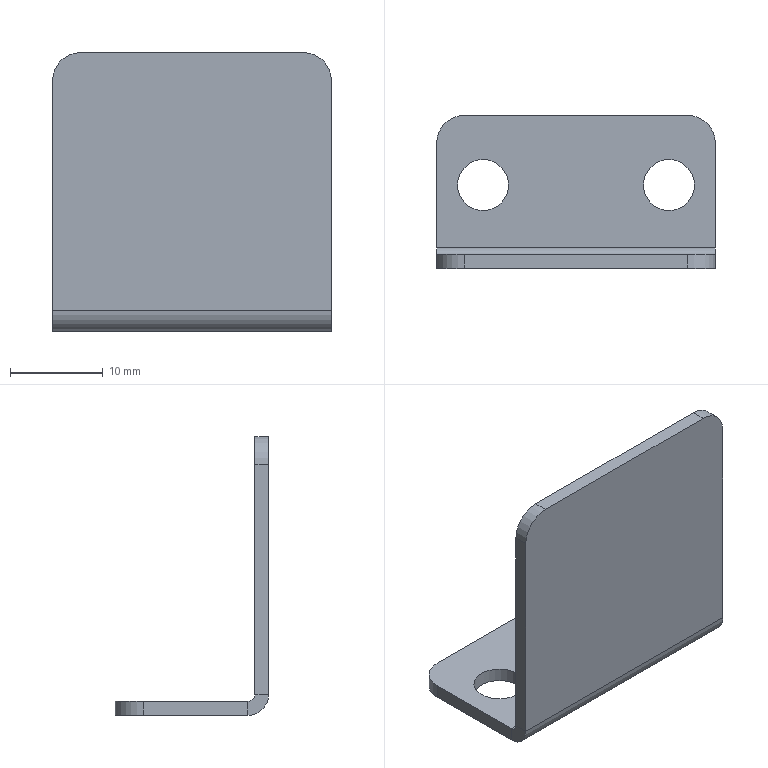Part | SolidWorks | features BaseBody 1 | 1 solid | 22 faces | box 30 x 16.5 x 30 mm | volume 1913 mm3 | plane 12 | cylinder 10 | commonest cylinder face diameters 5.5 x4 6 x4 1.473 x1 4.473 x1
STEP:
#1=CARTESIAN_POINT('',(-12.75,0.,-1.5));
#2=VERTEX_POINT('',#1);
#3=CARTESIAN_POINT('',(-7.25,0.,-1.5));
#4=VERTEX_POINT('',#3);
#5=CARTESIAN_POINT('',(-10.,0.,-1.5));
#6=DIRECTION('',(0.,0.,1.));
#7=DIRECTION('',(1.,0.,0.));
#8=AXIS2_PLACEMENT_3D('',#5,#6,#7);
#9=CIRCLE('',#8,2.75);
#10=EDGE_CURVE('',#2,#4,#9,.T.);
#11=ORIENTED_EDGE('',*,*,#10,.F.);
#12=CARTESIAN_POINT('',(-12.75,0.,0.));
#13=VERTEX_POINT('',#12);
#14=CARTESIAN_POINT('',(-12.75,0.,0.));
#15=DIRECTION('',(0.,0.,1.));
#16=VECTOR('',#15,1000.);
#17=LINE('',#14,#16);
#18=EDGE_CURVE('',#2,#13,#17,.T.);
#19=ORIENTED_EDGE('',*,*,#18,.T.);
#20=CARTESIAN_POINT('',(-7.25,0.,0.));
#21=VERTEX_POINT('',#20);
#22=CARTESIAN_POINT('',(-10.,0.,0.));
#23=DIRECTION('',(0.,0.,1.));
#24=DIRECTION('',(1.,0.,0.));
#25=AXIS2_PLACEMENT_3D('',#22,#23,#24);
#26=CIRCLE('',#25,2.75);
#27=EDGE_CURVE('',#13,#21,#26,.T.);
#28=ORIENTED_EDGE('',*,*,#27,.T.);
#29=CARTESIAN_POINT('',(-7.25,0.,0.));
#30=DIRECTION('',(0.,0.,1.));
#31=VECTOR('',#30,1000.);
#32=LINE('',#29,#31);
#33=EDGE_CURVE('',#4,#21,#32,.T.);
#34=ORIENTED_EDGE('',*,*,#33,.F.);
#35=EDGE_LOOP('',(#11,#19,#28,#34));
#36=FACE_OUTER_BOUND('',#35,.T.);
#37=CARTESIAN_POINT('',(-10.,0.,0.));
#38=DIRECTION('',(0.,0.,1.));
#39=DIRECTION('',(1.,0.,0.));
#40=AXIS2_PLACEMENT_3D('',#37,#38,#39);
#41=CYLINDRICAL_SURFACE('',#40,2.75);
#42=ADVANCED_FACE('',(#36),#41,.F.);
#43=CARTESIAN_POINT('',(7.25,0.,-1.5));
#44=VERTEX_POINT('',#43);
#45=CARTESIAN_POINT('',(12.75,0.,-1.5));
#46=VERTEX_POINT('',#45);
#47=CARTESIAN_POINT('',(10.,0.,-1.5));
#48=DIRECTION('',(0.,0.,1.));
#49=DIRECTION('',(1.,0.,0.));
#50=AXIS2_PLACEMENT_3D('',#47,#48,#49);
#51=CIRCLE('',#50,2.75);
#52=EDGE_CURVE('',#44,#46,#51,.T.);
#53=ORIENTED_EDGE('',*,*,#52,.F.);
#54=CARTESIAN_POINT('',(7.25,0.,0.));
#55=VERTEX_POINT('',#54);
#56=CARTESIAN_POINT('',(7.25,0.,0.));
#57=DIRECTION('',(0.,0.,1.));
#58=VECTOR('',#57,1000.);
#59=LINE('',#56,#58);
#60=EDGE_CURVE('',#44,#55,#59,.T.);
#61=ORIENTED_EDGE('',*,*,#60,.T.);
#62=CARTESIAN_POINT('',(12.75,0.,0.));
#63=VERTEX_POINT('',#62);
#64=CARTESIAN_POINT('',(10.,0.,0.));
#65=DIRECTION('',(0.,0.,1.));
#66=DIRECTION('',(1.,0.,0.));
#67=AXIS2_PLACEMENT_3D('',#64,#65,#66);
#68=CIRCLE('',#67,2.75);
#69=EDGE_CURVE('',#55,#63,#68,.T.);
#70=ORIENTED_EDGE('',*,*,#69,.T.);
#71=CARTESIAN_POINT('',(12.75,0.,0.));
#72=DIRECTION('',(0.,0.,1.));
#73=VECTOR('',#72,1000.);
#74=LINE('',#71,#73);
#75=EDGE_CURVE('',#46,#63,#74,.T.);
#76=ORIENTED_EDGE('',*,*,#75,.F.);
#77=EDGE_LOOP('',(#53,#61,#70,#76));
#78=FACE_OUTER_BOUND('',#77,.T.);
#79=CARTESIAN_POINT('',(10.,0.,0.));
#80=DIRECTION('',(0.,0.,1.));
#81=DIRECTION('',(1.,0.,0.));
#82=AXIS2_PLACEMENT_3D('',#79,#80,#81);
#83=CYLINDRICAL_SURFACE('',#82,2.75);
#84=ADVANCED_FACE('',(#78),#83,.F.);
#85=CARTESIAN_POINT('',(15.,-6.763,-1.5));
#86=VERTEX_POINT('',#85);
#87=CARTESIAN_POINT('',(15.,4.5,-1.5));
#88=VERTEX_POINT('',#87);
#89=CARTESIAN_POINT('',(15.,7.5,-1.5));
#90=DIRECTION('',(0.,1.,0.));
#91=VECTOR('',#90,1000.);
#92=LINE('',#89,#91);
#93=EDGE_CURVE('',#86,#88,#92,.T.);
#94=ORIENTED_EDGE('',*,*,#93,.T.);
#95=CARTESIAN_POINT('',(15.,4.5,0.));
#96=VERTEX_POINT('',#95);
#97=CARTESIAN_POINT('',(15.,4.5,-1.5));
#98=DIRECTION('',(0.,0.,1.));
#99=VECTOR('',#98,1000.);
#100=LINE('',#97,#99);
#101=EDGE_CURVE('',#88,#96,#100,.T.);
#102=ORIENTED_EDGE('',*,*,#101,.T.);
#103=CARTESIAN_POINT('',(15.,-6.763,0.));
#104=VERTEX_POINT('',#103);
#105=CARTESIAN_POINT('',(15.,7.5,0.));
#106=DIRECTION('',(0.,1.,0.));
#107=VECTOR('',#106,1000.);
#108=LINE('',#105,#107);
#109=EDGE_CURVE('',#104,#96,#108,.T.);
#110=ORIENTED_EDGE('',*,*,#109,.F.);
#111=CARTESIAN_POINT('',(15.,-6.763,0.));
#112=DIRECTION('',(0.,0.,-1.));
#113=VECTOR('',#112,1000.);
#114=LINE('',#111,#113);
#115=EDGE_CURVE('',#104,#86,#114,.T.);
#116=ORIENTED_EDGE('',*,*,#115,.T.);
#117=EDGE_LOOP('',(#94,#102,#110,#116));
#118=FACE_OUTER_BOUND('',#117,.T.);
#119=CARTESIAN_POINT('',(15.,7.5,-1.5));
#120=DIRECTION('',(1.,0.,0.));
#121=DIRECTION('',(0.,1.,0.));
#122=AXIS2_PLACEMENT_3D('',#119,#120,#121);
#123=PLANE('',#122);
#124=ADVANCED_FACE('',(#118),#123,.T.);
#125=CARTESIAN_POINT('',(-10.,0.,-1.5));
#126=DIRECTION('',(0.,0.,1.));
#127=DIRECTION('',(1.,0.,0.));
#128=AXIS2_PLACEMENT_3D('',#125,#126,#127);
#129=CIRCLE('',#128,2.75);
#130=EDGE_CURVE('',#4,#2,#129,.T.);
#131=ORIENTED_EDGE('',*,*,#130,.T.);
#132=ORIENTED_EDGE('',*,*,#10,.T.);
#133=EDGE_LOOP('',(#131,#132));
#134=FACE_BOUND('',#133,.T.);
#135=CARTESIAN_POINT('',(10.,0.,-1.5));
#136=DIRECTION('',(0.,0.,1.));
#137=DIRECTION('',(1.,0.,0.));
#138=AXIS2_PLACEMENT_3D('',#135,#136,#137);
#139=CIRCLE('',#138,2.75);
#140=EDGE_CURVE('',#46,#44,#139,.T.);
#141=ORIENTED_EDGE('',*,*,#140,.T.);
#142=ORIENTED_EDGE('',*,*,#52,.T.);
#143=EDGE_LOOP('',(#141,#142));
#144=FACE_BOUND('',#143,.T.);
#145=CARTESIAN_POINT('',(12.,7.5,-1.5));
#146=VERTEX_POINT('',#145);
#147=CARTESIAN_POINT('',(-12.,7.5,-1.5));
#148=VERTEX_POINT('',#147);
#149=CARTESIAN_POINT('',(15.,7.5,-1.5));
#150=DIRECTION('',(-1.,0.,0.));
#151=VECTOR('',#150,1000.);
#152=LINE('',#149,#151);
#153=EDGE_CURVE('',#146,#148,#152,.T.);
#154=ORIENTED_EDGE('',*,*,#153,.F.);
#155=CARTESIAN_POINT('',(12.,4.5,-1.5));
#156=DIRECTION('',(0.,0.,-1.));
#157=DIRECTION('',(-1.,0.,0.));
#158=AXIS2_PLACEMENT_3D('',#155,#156,#157);
#159=CIRCLE('',#158,3.);
#160=EDGE_CURVE('',#146,#88,#159,.T.);
#161=ORIENTED_EDGE('',*,*,#160,.T.);
#162=ORIENTED_EDGE('',*,*,#93,.F.);
#163=CARTESIAN_POINT('',(-15.,-6.763,-1.5));
#164=VERTEX_POINT('',#163);
#165=CARTESIAN_POINT('',(15.,-6.763,-1.5));
#166=DIRECTION('',(-1.,0.,0.));
#167=VECTOR('',#166,1000.);
#168=LINE('',#165,#167);
#169=EDGE_CURVE('',#86,#164,#168,.T.);
#170=ORIENTED_EDGE('',*,*,#169,.T.);
#171=CARTESIAN_POINT('',(-15.,4.5,-1.5));
#172=VERTEX_POINT('',#171);
#173=CARTESIAN_POINT('',(-15.,7.5,-1.5));
#174=DIRECTION('',(0.,-1.,0.));
#175=VECTOR('',#174,1000.);
#176=LINE('',#173,#175);
#177=EDGE_CURVE('',#172,#164,#176,.T.);
#178=ORIENTED_EDGE('',*,*,#177,.F.);
#179=CARTESIAN_POINT('',(-12.,4.5,-1.5));
#180=DIRECTION('',(0.,0.,-1.));
#181=DIRECTION('',(-1.,0.,0.));
#182=AXIS2_PLACEMENT_3D('',#179,#180,#181);
#183=CIRCLE('',#182,3.);
#184=EDGE_CURVE('',#172,#148,#183,.T.);
#185=ORIENTED_EDGE('',*,*,#184,.T.);
#186=EDGE_LOOP('',(#154,#161,#162,#170,#178,#185));
#187=FACE_OUTER_BOUND('',#186,.T.);
#188=CARTESIAN_POINT('',(0.,0.,-1.5));
#189=DIRECTION('',(0.,0.,-1.));
#190=DIRECTION('',(-1.,0.,0.));
#191=AXIS2_PLACEMENT_3D('',#188,#189,#190);
#192=PLANE('',#191);
#193=ADVANCED_FACE('',(#134,#144,#187),#192,.T.);
#194=CARTESIAN_POINT('',(-10.,0.,0.));
#195=DIRECTION('',(0.,0.,1.));
#196=DIRECTION('',(1.,0.,0.));
#197=AXIS2_PLACEMENT_3D('',#194,#195,#196);
#198=CIRCLE('',#197,2.75);
#199=EDGE_CURVE('',#21,#13,#198,.T.);
#200=ORIENTED_EDGE('',*,*,#199,.F.);
#201=ORIENTED_EDGE('',*,*,#27,.F.);
#202=EDGE_LOOP('',(#200,#201));
#203=FACE_BOUND('',#202,.T.);
#204=CARTESIAN_POINT('',(10.,0.,0.));
#205=DIRECTION('',(0.,0.,1.));
#206=DIRECTION('',(1.,0.,0.));
#207=AXIS2_PLACEMENT_3D('',#204,#205,#206);
#208=CIRCLE('',#207,2.75);
#209=EDGE_CURVE('',#63,#55,#208,.T.);
#210=ORIENTED_EDGE('',*,*,#209,.F.);
#211=ORIENTED_EDGE('',*,*,#69,.F.);
#212=EDGE_LOOP('',(#210,#211));
#213=FACE_BOUND('',#212,.T.);
#214=ORIENTED_EDGE('',*,*,#109,.T.);
#215=CARTESIAN_POINT('',(12.,7.5,0.));
#216=VERTEX_POINT('',#215);
#217=CARTESIAN_POINT('',(12.,4.5,0.));
#218=DIRECTION('',(0.,0.,1.));
#219=DIRECTION('',(-1.,0.,0.));
#220=AXIS2_PLACEMENT_3D('',#217,#218,#219);
#221=CIRCLE('',#220,3.);
#222=EDGE_CURVE('',#96,#216,#221,.T.);
#223=ORIENTED_EDGE('',*,*,#222,.T.);
#224=CARTESIAN_POINT('',(-12.,7.5,0.));
#225=VERTEX_POINT('',#224);
#226=CARTESIAN_POINT('',(15.,7.5,0.));
#227=DIRECTION('',(-1.,0.,0.));
#228=VECTOR('',#227,1000.);
#229=LINE('',#226,#228);
#230=EDGE_CURVE('',#216,#225,#229,.T.);
#231=ORIENTED_EDGE('',*,*,#230,.T.);
#232=CARTESIAN_POINT('',(-15.,4.5,0.));
#233=VERTEX_POINT('',#232);
#234=CARTESIAN_POINT('',(-12.,4.5,0.));
#235=DIRECTION('',(0.,0.,1.));
#236=DIRECTION('',(-1.,0.,0.));
#237=AXIS2_PLACEMENT_3D('',#234,#235,#236);
#238=CIRCLE('',#237,3.);
#239=EDGE_CURVE('',#225,#233,#238,.T.);
#240=ORIENTED_EDGE('',*,*,#239,.T.);
#241=CARTESIAN_POINT('',(-15.,-6.763,0.));
#242=VERTEX_POINT('',#241);
#243=CARTESIAN_POINT('',(-15.,7.5,0.));
#244=DIRECTION('',(0.,-1.,0.));
#245=VECTOR('',#244,1000.);
#246=LINE('',#243,#245);
#247=EDGE_CURVE('',#233,#242,#246,.T.);
#248=ORIENTED_EDGE('',*,*,#247,.T.);
#249=CARTESIAN_POINT('',(15.,-6.763,0.));
#250=DIRECTION('',(-1.,0.,0.));
#251=VECTOR('',#250,1000.);
#252=LINE('',#249,#251);
#253=EDGE_CURVE('',#104,#242,#252,.T.);
#254=ORIENTED_EDGE('',*,*,#253,.F.);
#255=EDGE_LOOP('',(#214,#223,#231,#240,#248,#254));
#256=FACE_OUTER_BOUND('',#255,.T.);
#257=CARTESIAN_POINT('',(0.,0.,0.));
#258=DIRECTION('',(0.,0.,-1.));
#259=DIRECTION('',(-1.,0.,0.));
#260=AXIS2_PLACEMENT_3D('',#257,#258,#259);
#261=PLANE('',#260);
#262=ADVANCED_FACE('',(#203,#213,#256),#261,.F.);
#263=ORIENTED_EDGE('',*,*,#247,.F.);
#264=CARTESIAN_POINT('',(-15.,4.5,-1.5));
#265=DIRECTION('',(0.,0.,-1.));
#266=VECTOR('',#265,1000.);
#267=LINE('',#264,#266);
#268=EDGE_CURVE('',#233,#172,#267,.T.);
#269=ORIENTED_EDGE('',*,*,#268,.T.);
#270=ORIENTED_EDGE('',*,*,#177,.T.);
#271=CARTESIAN_POINT('',(-15.,-6.763,0.));
#272=DIRECTION('',(0.,0.,-1.));
#273=VECTOR('',#272,1000.);
#274=LINE('',#271,#273);
#275=EDGE_CURVE('',#242,#164,#274,.T.);
#276=ORIENTED_EDGE('',*,*,#275,.F.);
#277=EDGE_LOOP('',(#263,#269,#270,#276));
#278=FACE_OUTER_BOUND('',#277,.T.);
#279=CARTESIAN_POINT('',(-15.,7.5,-1.5));
#280=DIRECTION('',(-1.,0.,0.));
#281=DIRECTION('',(0.,-1.,0.));
#282=AXIS2_PLACEMENT_3D('',#279,#280,#281);
#283=PLANE('',#282);
#284=ADVANCED_FACE('',(#278),#283,.T.);
#285=ORIENTED_EDGE('',*,*,#230,.F.);
#286=CARTESIAN_POINT('',(12.,7.5,-1.5));
#287=DIRECTION('',(0.,0.,-1.));
#288=VECTOR('',#287,1000.);
#289=LINE('',#286,#288);
#290=EDGE_CURVE('',#216,#146,#289,.T.);
#291=ORIENTED_EDGE('',*,*,#290,.T.);
#292=ORIENTED_EDGE('',*,*,#153,.T.);
#293=CARTESIAN_POINT('',(-12.,7.5,-1.5));
#294=DIRECTION('',(0.,0.,1.));
#295=VECTOR('',#294,1000.);
#296=LINE('',#293,#295);
#297=EDGE_CURVE('',#148,#225,#296,.T.);
#298=ORIENTED_EDGE('',*,*,#297,.T.);
#299=EDGE_LOOP('',(#285,#291,#292,#298));
#300=FACE_OUTER_BOUND('',#299,.T.);
#301=CARTESIAN_POINT('',(15.,7.5,-1.5));
#302=DIRECTION('',(0.,1.,0.));
#303=DIRECTION('',(-1.,0.,0.));
#304=AXIS2_PLACEMENT_3D('',#301,#302,#303);
#305=PLANE('',#304);
#306=ADVANCED_FACE('',(#300),#305,.T.);
#307=CARTESIAN_POINT('',(-15.,-7.5,0.7366));
#308=VERTEX_POINT('',#307);
#309=CARTESIAN_POINT('',(-15.,-9.,0.7366));
#310=VERTEX_POINT('',#309);
#311=CARTESIAN_POINT('',(-15.,-7.5,0.7366));
#312=DIRECTION('',(0.,-1.,0.));
#313=VECTOR('',#312,1000.);
#314=LINE('',#311,#313);
#315=EDGE_CURVE('',#308,#310,#314,.T.);
#316=ORIENTED_EDGE('',*,*,#315,.F.);
#317=CARTESIAN_POINT('',(-15.,-6.763,0.7366));
#318=DIRECTION('',(-1.,0.,0.));
#319=DIRECTION('',(0.,0.,-1.));
#320=AXIS2_PLACEMENT_3D('',#317,#318,#319);
#321=CIRCLE('',#320,0.7366);
#322=EDGE_CURVE('',#242,#308,#321,.T.);
#323=ORIENTED_EDGE('',*,*,#322,.F.);
#324=ORIENTED_EDGE('',*,*,#275,.T.);
#325=CARTESIAN_POINT('',(-15.,-6.763,0.7366));
#326=DIRECTION('',(-1.,0.,0.));
#327=DIRECTION('',(0.,0.,-1.));
#328=AXIS2_PLACEMENT_3D('',#325,#326,#327);
#329=CIRCLE('',#328,2.237);
#330=EDGE_CURVE('',#164,#310,#329,.T.);
#331=ORIENTED_EDGE('',*,*,#330,.T.);
#332=EDGE_LOOP('',(#316,#323,#324,#331));
#333=FACE_OUTER_BOUND('',#332,.T.);
#334=CARTESIAN_POINT('',(-15.,-6.763,0.7366));
#335=DIRECTION('',(-1.,0.,0.));
#336=DIRECTION('',(0.,0.,1.));
#337=AXIS2_PLACEMENT_3D('',#334,#335,#336);
#338=PLANE('',#337);
#339=ADVANCED_FACE('',(#333),#338,.T.);
#340=CARTESIAN_POINT('',(15.,-7.5,0.7366));
#341=VERTEX_POINT('',#340);
#342=CARTESIAN_POINT('',(15.,-6.763,0.7366));
#343=DIRECTION('',(1.,0.,0.));
#344=DIRECTION('',(0.,0.,-1.));
#345=AXIS2_PLACEMENT_3D('',#342,#343,#344);
#346=CIRCLE('',#345,0.7366);
#347=EDGE_CURVE('',#341,#104,#346,.T.);
#348=ORIENTED_EDGE('',*,*,#347,.F.);
#349=CARTESIAN_POINT('',(15.,-9.,0.7366));
#350=VERTEX_POINT('',#349);
#351=CARTESIAN_POINT('',(15.,-7.5,0.7366));
#352=DIRECTION('',(0.,-1.,0.));
#353=VECTOR('',#352,1000.);
#354=LINE('',#351,#353);
#355=EDGE_CURVE('',#341,#350,#354,.T.);
#356=ORIENTED_EDGE('',*,*,#355,.T.);
#357=CARTESIAN_POINT('',(15.,-6.763,0.7366));
#358=DIRECTION('',(1.,0.,0.));
#359=DIRECTION('',(0.,0.,-1.));
#360=AXIS2_PLACEMENT_3D('',#357,#358,#359);
#361=CIRCLE('',#360,2.237);
#362=EDGE_CURVE('',#350,#86,#361,.T.);
#363=ORIENTED_EDGE('',*,*,#362,.T.);
#364=ORIENTED_EDGE('',*,*,#115,.F.);
#365=EDGE_LOOP('',(#348,#356,#363,#364));
#366=FACE_OUTER_BOUND('',#365,.T.);
#367=CARTESIAN_POINT('',(15.,-6.763,0.7366));
#368=DIRECTION('',(-1.,0.,0.));
#369=DIRECTION('',(0.,0.,1.));
#370=AXIS2_PLACEMENT_3D('',#367,#368,#369);
#371=PLANE('',#370);
#372=ADVANCED_FACE('',(#366),#371,.F.);
#373=ORIENTED_EDGE('',*,*,#169,.F.);
#374=ORIENTED_EDGE('',*,*,#362,.F.);
#375=CARTESIAN_POINT('',(0.,-9.,0.7366));
#376=DIRECTION('',(1.,0.,0.));
#377=VECTOR('',#376,1000.);
#378=LINE('',#375,#377);
#379=EDGE_CURVE('',#310,#350,#378,.T.);
#380=ORIENTED_EDGE('',*,*,#379,.F.);
#381=ORIENTED_EDGE('',*,*,#330,.F.);
#382=EDGE_LOOP('',(#373,#374,#380,#381));
#383=FACE_OUTER_BOUND('',#382,.T.);
#384=CARTESIAN_POINT('',(15.,-6.763,0.7366));
#385=DIRECTION('',(1.,0.,0.));
#386=DIRECTION('',(0.,-1.,0.));
#387=AXIS2_PLACEMENT_3D('',#384,#385,#386);
#388=CYLINDRICAL_SURFACE('',#387,2.237);
#389=ADVANCED_FACE('',(#383),#388,.T.);
#390=ORIENTED_EDGE('',*,*,#253,.T.);
#391=ORIENTED_EDGE('',*,*,#322,.T.);
#392=CARTESIAN_POINT('',(-15.,-7.5,0.7366));
#393=DIRECTION('',(1.,0.,0.));
#394=VECTOR('',#393,1000.);
#395=LINE('',#392,#394);
#396=EDGE_CURVE('',#308,#341,#395,.T.);
#397=ORIENTED_EDGE('',*,*,#396,.T.);
#398=ORIENTED_EDGE('',*,*,#347,.T.);
#399=EDGE_LOOP('',(#390,#391,#397,#398));
#400=FACE_OUTER_BOUND('',#399,.T.);
#401=CARTESIAN_POINT('',(15.,-6.763,0.7366));
#402=DIRECTION('',(1.,0.,0.));
#403=DIRECTION('',(0.,-1.,0.));
#404=AXIS2_PLACEMENT_3D('',#401,#402,#403);
#405=CYLINDRICAL_SURFACE('',#404,0.7366);
#406=ADVANCED_FACE('',(#400),#405,.F.);
#407=CARTESIAN_POINT('',(15.,-7.5,25.5));
#408=VERTEX_POINT('',#407);
#409=CARTESIAN_POINT('',(15.,-7.5,0.));
#410=DIRECTION('',(0.,0.,-1.));
#411=VECTOR('',#410,1000.);
#412=LINE('',#409,#411);
#413=EDGE_CURVE('',#408,#341,#412,.T.);
#414=ORIENTED_EDGE('',*,*,#413,.F.);
#415=CARTESIAN_POINT('',(15.,-9.,25.5));
#416=VERTEX_POINT('',#415);
#417=CARTESIAN_POINT('',(15.,-9.,25.5));
#418=DIRECTION('',(0.,-1.,0.));
#419=VECTOR('',#418,1000.);
#420=LINE('',#417,#419);
#421=EDGE_CURVE('',#408,#416,#420,.T.);
#422=ORIENTED_EDGE('',*,*,#421,.T.);
#423=CARTESIAN_POINT('',(15.,-9.,0.));
#424=DIRECTION('',(0.,0.,-1.));
#425=VECTOR('',#424,1000.);
#426=LINE('',#423,#425);
#427=EDGE_CURVE('',#416,#350,#426,.T.);
#428=ORIENTED_EDGE('',*,*,#427,.T.);
#429=ORIENTED_EDGE('',*,*,#355,.F.);
#430=EDGE_LOOP('',(#414,#422,#428,#429));
#431=FACE_OUTER_BOUND('',#430,.T.);
#432=CARTESIAN_POINT('',(15.,-9.,0.));
#433=DIRECTION('',(1.,0.,0.));
#434=DIRECTION('',(0.,1.,0.));
#435=AXIS2_PLACEMENT_3D('',#432,#433,#434);
#436=PLANE('',#435);
#437=ADVANCED_FACE('',(#431),#436,.T.);
#438=CARTESIAN_POINT('',(-15.,-9.,25.5));
#439=VERTEX_POINT('',#438);
#440=CARTESIAN_POINT('',(-15.,-9.,28.5));
#441=DIRECTION('',(0.,0.,1.));
#442=VECTOR('',#441,1000.);
#443=LINE('',#440,#442);
#444=EDGE_CURVE('',#310,#439,#443,.T.);
#445=ORIENTED_EDGE('',*,*,#444,.T.);
#446=CARTESIAN_POINT('',(-15.,-7.5,25.5));
#447=VERTEX_POINT('',#446);
#448=CARTESIAN_POINT('',(-15.,-9.,25.5));
#449=DIRECTION('',(0.,1.,0.));
#450=VECTOR('',#449,1000.);
#451=LINE('',#448,#450);
#452=EDGE_CURVE('',#439,#447,#451,.T.);
#453=ORIENTED_EDGE('',*,*,#452,.T.);
#454=CARTESIAN_POINT('',(-15.,-7.5,28.5));
#455=DIRECTION('',(0.,0.,1.));
#456=VECTOR('',#455,1000.);
#457=LINE('',#454,#456);
#458=EDGE_CURVE('',#308,#447,#457,.T.);
#459=ORIENTED_EDGE('',*,*,#458,.F.);
#460=ORIENTED_EDGE('',*,*,#315,.T.);
#461=EDGE_LOOP('',(#445,#453,#459,#460));
#462=FACE_OUTER_BOUND('',#461,.T.);
#463=CARTESIAN_POINT('',(-15.,-9.,28.5));
#464=DIRECTION('',(-1.,0.,0.));
#465=DIRECTION('',(0.,-1.,0.));
#466=AXIS2_PLACEMENT_3D('',#463,#464,#465);
#467=PLANE('',#466);
#468=ADVANCED_FACE('',(#462),#467,.T.);
#469=ORIENTED_EDGE('',*,*,#427,.F.);
#470=CARTESIAN_POINT('',(12.,-9.,28.5));
#471=VERTEX_POINT('',#470);
#472=CARTESIAN_POINT('',(12.,-9.,25.5));
#473=DIRECTION('',(0.,-1.,0.));
#474=DIRECTION('',(0.,0.,-1.));
#475=AXIS2_PLACEMENT_3D('',#472,#473,#474);
#476=CIRCLE('',#475,3.);
#477=EDGE_CURVE('',#416,#471,#476,.T.);
#478=ORIENTED_EDGE('',*,*,#477,.T.);
#479=CARTESIAN_POINT('',(-12.,-9.,28.5));
#480=VERTEX_POINT('',#479);
#481=CARTESIAN_POINT('',(15.,-9.,28.5));
#482=DIRECTION('',(1.,0.,0.));
#483=VECTOR('',#482,1000.);
#484=LINE('',#481,#483);
#485=EDGE_CURVE('',#480,#471,#484,.T.);
#486=ORIENTED_EDGE('',*,*,#485,.F.);
#487=CARTESIAN_POINT('',(-12.,-9.,25.5));
#488=DIRECTION('',(0.,-1.,0.));
#489=DIRECTION('',(0.,0.,-1.));
#490=AXIS2_PLACEMENT_3D('',#487,#488,#489);
#491=CIRCLE('',#490,3.);
#492=EDGE_CURVE('',#480,#439,#491,.T.);
#493=ORIENTED_EDGE('',*,*,#492,.T.);
#494=ORIENTED_EDGE('',*,*,#444,.F.);
#495=ORIENTED_EDGE('',*,*,#379,.T.);
#496=EDGE_LOOP('',(#469,#478,#486,#493,#494,#495));
#497=FACE_OUTER_BOUND('',#496,.T.);
#498=CARTESIAN_POINT('',(0.,-9.,0.));
#499=DIRECTION('',(0.,-1.,0.));
#500=DIRECTION('',(0.,0.,-1.));
#501=AXIS2_PLACEMENT_3D('',#498,#499,#500);
#502=PLANE('',#501);
#503=ADVANCED_FACE('',(#497),#502,.T.);
#504=CARTESIAN_POINT('',(-12.,-7.5,28.5));
#505=VERTEX_POINT('',#504);
#506=CARTESIAN_POINT('',(12.,-7.5,28.5));
#507=VERTEX_POINT('',#506);
#508=CARTESIAN_POINT('',(15.,-7.5,28.5));
#509=DIRECTION('',(1.,0.,0.));
#510=VECTOR('',#509,1000.);
#511=LINE('',#508,#510);
#512=EDGE_CURVE('',#505,#507,#511,.T.);
#513=ORIENTED_EDGE('',*,*,#512,.T.);
#514=CARTESIAN_POINT('',(12.,-7.5,25.5));
#515=DIRECTION('',(0.,1.,0.));
#516=DIRECTION('',(0.,0.,-1.));
#517=AXIS2_PLACEMENT_3D('',#514,#515,#516);
#518=CIRCLE('',#517,3.);
#519=EDGE_CURVE('',#507,#408,#518,.T.);
#520=ORIENTED_EDGE('',*,*,#519,.T.);
#521=ORIENTED_EDGE('',*,*,#413,.T.);
#522=ORIENTED_EDGE('',*,*,#396,.F.);
#523=ORIENTED_EDGE('',*,*,#458,.T.);
#524=CARTESIAN_POINT('',(-12.,-7.5,25.5));
#525=DIRECTION('',(0.,1.,0.));
#526=DIRECTION('',(0.,0.,-1.));
#527=AXIS2_PLACEMENT_3D('',#524,#525,#526);
#528=CIRCLE('',#527,3.);
#529=EDGE_CURVE('',#447,#505,#528,.T.);
#530=ORIENTED_EDGE('',*,*,#529,.T.);
#531=EDGE_LOOP('',(#513,#520,#521,#522,#523,#530));
#532=FACE_OUTER_BOUND('',#531,.T.);
#533=CARTESIAN_POINT('',(0.,-7.5,0.));
#534=DIRECTION('',(0.,-1.,0.));
#535=DIRECTION('',(0.,0.,-1.));
#536=AXIS2_PLACEMENT_3D('',#533,#534,#535);
#537=PLANE('',#536);
#538=ADVANCED_FACE('',(#532),#537,.F.);
#539=ORIENTED_EDGE('',*,*,#485,.T.);
#540=CARTESIAN_POINT('',(12.,-9.,28.5));
#541=DIRECTION('',(0.,1.,0.));
#542=VECTOR('',#541,1000.);
#543=LINE('',#540,#542);
#544=EDGE_CURVE('',#471,#507,#543,.T.);
#545=ORIENTED_EDGE('',*,*,#544,.T.);
#546=ORIENTED_EDGE('',*,*,#512,.F.);
#547=CARTESIAN_POINT('',(-12.,-9.,28.5));
#548=DIRECTION('',(0.,-1.,0.));
#549=VECTOR('',#548,1000.);
#550=LINE('',#547,#549);
#551=EDGE_CURVE('',#505,#480,#550,.T.);
#552=ORIENTED_EDGE('',*,*,#551,.T.);
#553=EDGE_LOOP('',(#539,#545,#546,#552));
#554=FACE_OUTER_BOUND('',#553,.T.);
#555=CARTESIAN_POINT('',(15.,-9.,28.5));
#556=DIRECTION('',(0.,0.,1.));
#557=DIRECTION('',(0.,-1.,0.));
#558=AXIS2_PLACEMENT_3D('',#555,#556,#557);
#559=PLANE('',#558);
#560=ADVANCED_FACE('',(#554),#559,.T.);
#561=ORIENTED_EDGE('',*,*,#477,.F.);
#562=ORIENTED_EDGE('',*,*,#421,.F.);
#563=ORIENTED_EDGE('',*,*,#519,.F.);
#564=ORIENTED_EDGE('',*,*,#544,.F.);
#565=EDGE_LOOP('',(#561,#562,#563,#564));
#566=FACE_OUTER_BOUND('',#565,.T.);
#567=CARTESIAN_POINT('',(12.,-9.,25.5));
#568=DIRECTION('',(0.,1.,0.));
#569=DIRECTION('',(0.,0.,1.));
#570=AXIS2_PLACEMENT_3D('',#567,#568,#569);
#571=CYLINDRICAL_SURFACE('',#570,3.);
#572=ADVANCED_FACE('',(#566),#571,.T.);
#573=ORIENTED_EDGE('',*,*,#492,.F.);
#574=ORIENTED_EDGE('',*,*,#551,.F.);
#575=ORIENTED_EDGE('',*,*,#529,.F.);
#576=ORIENTED_EDGE('',*,*,#452,.F.);
#577=EDGE_LOOP('',(#573,#574,#575,#576));
#578=FACE_OUTER_BOUND('',#577,.T.);
#579=CARTESIAN_POINT('',(-12.,-9.,25.5));
#580=DIRECTION('',(0.,1.,0.));
#581=DIRECTION('',(0.,0.,1.));
#582=AXIS2_PLACEMENT_3D('',#579,#580,#581);
#583=CYLINDRICAL_SURFACE('',#582,3.);
#584=ADVANCED_FACE('',(#578),#583,.T.);
#585=ORIENTED_EDGE('',*,*,#160,.F.);
#586=ORIENTED_EDGE('',*,*,#290,.F.);
#587=ORIENTED_EDGE('',*,*,#222,.F.);
#588=ORIENTED_EDGE('',*,*,#101,.F.);
#589=EDGE_LOOP('',(#585,#586,#587,#588));
#590=FACE_OUTER_BOUND('',#589,.T.);
#591=CARTESIAN_POINT('',(12.,4.5,-1.5));
#592=DIRECTION('',(0.,0.,1.));
#593=DIRECTION('',(1.,0.,0.));
#594=AXIS2_PLACEMENT_3D('',#591,#592,#593);
#595=CYLINDRICAL_SURFACE('',#594,3.);
#596=ADVANCED_FACE('',(#590),#595,.T.);
#597=ORIENTED_EDGE('',*,*,#184,.F.);
#598=ORIENTED_EDGE('',*,*,#268,.F.);
#599=ORIENTED_EDGE('',*,*,#239,.F.);
#600=ORIENTED_EDGE('',*,*,#297,.F.);
#601=EDGE_LOOP('',(#597,#598,#599,#600));
#602=FACE_OUTER_BOUND('',#601,.T.);
#603=CARTESIAN_POINT('',(-12.,4.5,-1.5));
#604=DIRECTION('',(0.,0.,1.));
#605=DIRECTION('',(1.,0.,0.));
#606=AXIS2_PLACEMENT_3D('',#603,#604,#605);
#607=CYLINDRICAL_SURFACE('',#606,3.);
#608=ADVANCED_FACE('',(#602),#607,.T.);
#609=ORIENTED_EDGE('',*,*,#60,.F.);
#610=ORIENTED_EDGE('',*,*,#140,.F.);
#611=ORIENTED_EDGE('',*,*,#75,.T.);
#612=ORIENTED_EDGE('',*,*,#209,.T.);
#613=EDGE_LOOP('',(#609,#610,#611,#612));
#614=FACE_OUTER_BOUND('',#613,.T.);
#615=CARTESIAN_POINT('',(10.,0.,0.));
#616=DIRECTION('',(0.,0.,1.));
#617=DIRECTION('',(1.,0.,0.));
#618=AXIS2_PLACEMENT_3D('',#615,#616,#617);
#619=CYLINDRICAL_SURFACE('',#618,2.75);
#620=ADVANCED_FACE('',(#614),#619,.F.);
#621=ORIENTED_EDGE('',*,*,#18,.F.);
#622=ORIENTED_EDGE('',*,*,#130,.F.);
#623=ORIENTED_EDGE('',*,*,#33,.T.);
#624=ORIENTED_EDGE('',*,*,#199,.T.);
#625=EDGE_LOOP('',(#621,#622,#623,#624));
#626=FACE_OUTER_BOUND('',#625,.T.);
#627=CARTESIAN_POINT('',(-10.,0.,0.));
#628=DIRECTION('',(0.,0.,1.));
#629=DIRECTION('',(1.,0.,0.));
#630=AXIS2_PLACEMENT_3D('',#627,#628,#629);
#631=CYLINDRICAL_SURFACE('',#630,2.75);
#632=ADVANCED_FACE('',(#626),#631,.F.);
#633=CLOSED_SHELL('',(#42,#84,#124,#193,#262,#284,#306,#339,#372,#389,#406,#437,#468,#503,#538,#560,#572,#584,#596,#608,#620,#632));
#634=MANIFOLD_SOLID_BREP('',#633);
#635=CARTESIAN_POINT('',(0.,0.,0.));
#636=DIRECTION('',(0.,0.,1.));
#637=DIRECTION('',(1.,0.,0.));
#638=AXIS2_PLACEMENT_3D('',#635,#636,#637);
#639=(LENGTH_UNIT()NAMED_UNIT(*)SI_UNIT(.MILLI.,.METRE.));
#640=UNCERTAINTY_MEASURE_WITH_UNIT(LENGTH_MEASURE(0.00001),#639,'','');
#641=(NAMED_UNIT(*)PLANE_ANGLE_UNIT()SI_UNIT($,.RADIAN.));
#642=(NAMED_UNIT(*)SI_UNIT($,.STERADIAN.)SOLID_ANGLE_UNIT());
#643=(GEOMETRIC_REPRESENTATION_CONTEXT(3)GLOBAL_UNCERTAINTY_ASSIGNED_CONTEXT((#640))GLOBAL_UNIT_ASSIGNED_CONTEXT((#639,#641,#642))REPRESENTATION_CONTEXT('',''));
#644=ADVANCED_BREP_SHAPE_REPRESENTATION('',(#634,#638),#643);